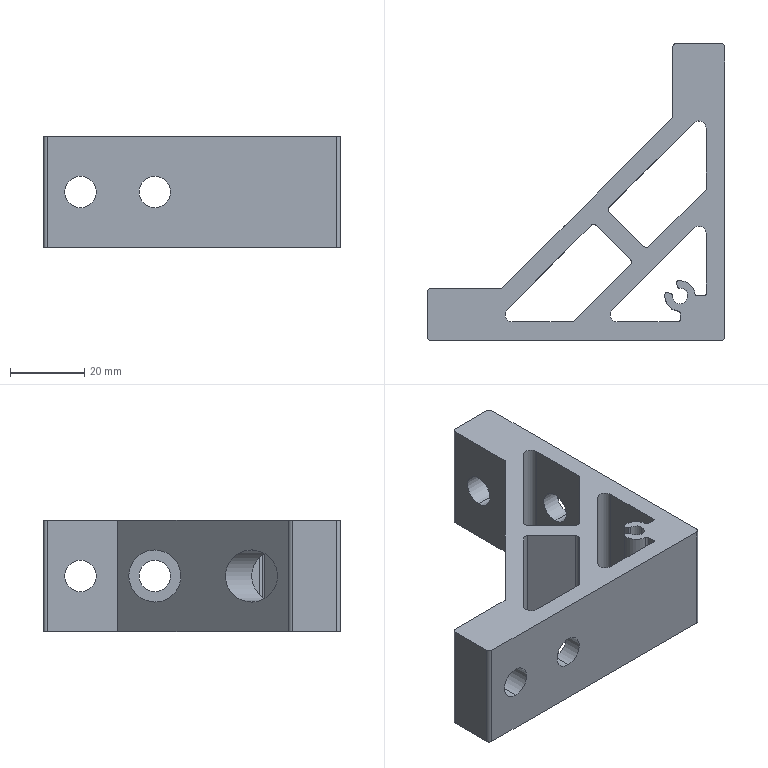Part | SolidWorks | features BaseBody 1 | 1 solid | 65 faces | box 80 x 80 x 30 mm | volume 51823 mm3 | cylinder 41 | plane 24 | commonest cylinder face diameters 2 x10 1 x9 8.5 x8 4 x5 14 x4 4.2 x3